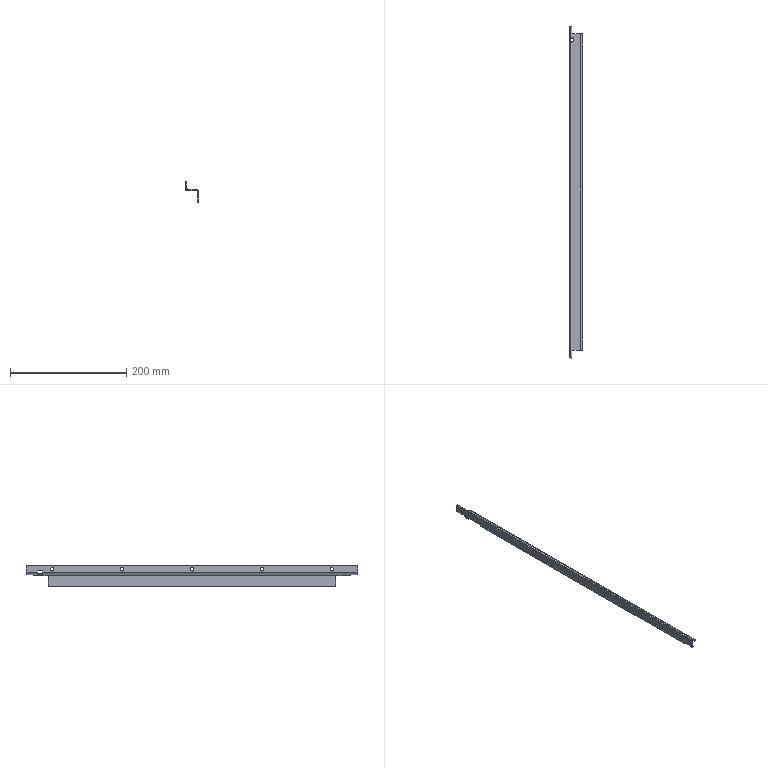Part | NX | features solid 2 | 1 solid | 44 faces | box 22 x 570 x 35 mm | volume 55640 mm3 | plane 26 | cylinder 18 | commonest cylinder face diameters 6 x12 4 x3 8 x3
STEP:
#1=CARTESIAN_POINT('',(-1103.5,-759.5,940.));
#2=VERTEX_POINT('',#1);
#3=CARTESIAN_POINT('',(-1103.5,-759.5,942.));
#4=VERTEX_POINT('',#3);
#5=CARTESIAN_POINT('',(-1103.5,-759.5,940.));
#6=DIRECTION('',(0.,0.,1.));
#7=VECTOR('',#6,1000.);
#8=LINE('',#5,#7);
#9=EDGE_CURVE('',#2,#4,#8,.T.);
#10=ORIENTED_EDGE('',*,*,#9,.F.);
#11=CARTESIAN_POINT('',(-1103.5,-765.5,940.));
#12=VERTEX_POINT('',#11);
#13=CARTESIAN_POINT('',(-1103.5,-762.5,940.));
#14=DIRECTION('',(0.,0.,1.));
#15=DIRECTION('',(0.,-1.,0.));
#16=AXIS2_PLACEMENT_3D('',#13,#14,#15);
#17=CIRCLE('',#16,3.);
#18=EDGE_CURVE('',#12,#2,#17,.T.);
#19=ORIENTED_EDGE('',*,*,#18,.F.);
#20=CARTESIAN_POINT('',(-1103.5,-765.5,942.));
#21=VERTEX_POINT('',#20);
#22=CARTESIAN_POINT('',(-1103.5,-765.5,940.));
#23=DIRECTION('',(0.,0.,1.));
#24=VECTOR('',#23,1000.);
#25=LINE('',#22,#24);
#26=EDGE_CURVE('',#21,#12,#25,.F.);
#27=ORIENTED_EDGE('',*,*,#26,.F.);
#28=CARTESIAN_POINT('',(-1103.5,-762.5,942.));
#29=DIRECTION('',(0.,0.,1.));
#30=DIRECTION('',(-1.,0.,0.));
#31=AXIS2_PLACEMENT_3D('',#28,#29,#30);
#32=CIRCLE('',#31,3.);
#33=EDGE_CURVE('',#21,#4,#32,.T.);
#34=ORIENTED_EDGE('',*,*,#33,.T.);
#35=EDGE_LOOP('',(#10,#19,#27,#34));
#36=FACE_BOUND('',#35,.T.);
#37=CARTESIAN_POINT('',(-1103.5,-762.5,940.));
#38=DIRECTION('',(0.,0.,1.));
#39=DIRECTION('',(0.,-1.,0.));
#40=AXIS2_PLACEMENT_3D('',#37,#38,#39);
#41=CYLINDRICAL_SURFACE('',#40,3.);
#42=ADVANCED_FACE('',(#36),#41,.F.);
#43=CARTESIAN_POINT('',(-1104.,-758.,940.));
#44=VERTEX_POINT('',#43);
#45=CARTESIAN_POINT('',(-1104.,-758.1,940.));
#46=VERTEX_POINT('',#45);
#47=CARTESIAN_POINT('',(-1104.,-758.1,940.));
#48=DIRECTION('',(0.,-1.,0.));
#49=VECTOR('',#48,1000.);
#50=LINE('',#47,#49);
#51=EDGE_CURVE('',#44,#46,#50,.T.);
#52=ORIENTED_EDGE('',*,*,#51,.T.);
#53=CARTESIAN_POINT('',(-1104.,-758.1,942.));
#54=VERTEX_POINT('',#53);
#55=CARTESIAN_POINT('',(-1104.,-758.1,942.));
#56=DIRECTION('',(0.,0.,-1.));
#57=VECTOR('',#56,1000.);
#58=LINE('',#55,#57);
#59=EDGE_CURVE('',#54,#46,#58,.T.);
#60=ORIENTED_EDGE('',*,*,#59,.F.);
#61=CARTESIAN_POINT('',(-1104.,-758.,942.));
#62=VERTEX_POINT('',#61);
#63=CARTESIAN_POINT('',(-1104.,-758.1,942.));
#64=DIRECTION('',(0.,-1.,0.));
#65=VECTOR('',#64,1000.);
#66=LINE('',#63,#65);
#67=EDGE_CURVE('',#62,#54,#66,.T.);
#68=ORIENTED_EDGE('',*,*,#67,.F.);
#69=CARTESIAN_POINT('',(-1104.,-758.,942.));
#70=DIRECTION('',(0.,0.,-1.));
#71=VECTOR('',#70,1000.);
#72=LINE('',#69,#71);
#73=EDGE_CURVE('',#62,#44,#72,.T.);
#74=ORIENTED_EDGE('',*,*,#73,.T.);
#75=EDGE_LOOP('',(#52,#60,#68,#74));
#76=FACE_BOUND('',#75,.T.);
#77=CARTESIAN_POINT('',(-1104.,-758.1,942.));
#78=DIRECTION('',(1.,0.,0.));
#79=DIRECTION('',(0.,0.,-1.));
#80=AXIS2_PLACEMENT_3D('',#77,#78,#79);
#81=PLANE('',#80);
#82=ADVANCED_FACE('',(#76),#81,.F.);
#83=CARTESIAN_POINT('',(-1104.,-767.9,940.));
#84=VERTEX_POINT('',#83);
#85=CARTESIAN_POINT('',(-1104.,-768.,940.));
#86=VERTEX_POINT('',#85);
#87=CARTESIAN_POINT('',(-1104.,-768.,940.));
#88=DIRECTION('',(0.,-1.,0.));
#89=VECTOR('',#88,1000.);
#90=LINE('',#87,#89);
#91=EDGE_CURVE('',#84,#86,#90,.T.);
#92=ORIENTED_EDGE('',*,*,#91,.T.);
#93=CARTESIAN_POINT('',(-1104.,-768.,942.));
#94=VERTEX_POINT('',#93);
#95=CARTESIAN_POINT('',(-1104.,-768.,942.));
#96=DIRECTION('',(0.,0.,-1.));
#97=VECTOR('',#96,1000.);
#98=LINE('',#95,#97);
#99=EDGE_CURVE('',#94,#86,#98,.T.);
#100=ORIENTED_EDGE('',*,*,#99,.F.);
#101=CARTESIAN_POINT('',(-1104.,-767.9,942.));
#102=VERTEX_POINT('',#101);
#103=CARTESIAN_POINT('',(-1104.,-768.,942.));
#104=DIRECTION('',(0.,-1.,0.));
#105=VECTOR('',#104,1000.);
#106=LINE('',#103,#105);
#107=EDGE_CURVE('',#102,#94,#106,.T.);
#108=ORIENTED_EDGE('',*,*,#107,.F.);
#109=CARTESIAN_POINT('',(-1104.,-767.9,942.));
#110=DIRECTION('',(0.,0.,-1.));
#111=VECTOR('',#110,1000.);
#112=LINE('',#109,#111);
#113=EDGE_CURVE('',#102,#84,#112,.T.);
#114=ORIENTED_EDGE('',*,*,#113,.T.);
#115=EDGE_LOOP('',(#92,#100,#108,#114));
#116=FACE_BOUND('',#115,.T.);
#117=CARTESIAN_POINT('',(-1104.,-768.,942.));
#118=DIRECTION('',(1.,0.,0.));
#119=DIRECTION('',(0.,0.,-1.));
#120=AXIS2_PLACEMENT_3D('',#117,#118,#119);
#121=PLANE('',#120);
#122=ADVANCED_FACE('',(#116),#121,.F.);
#123=CARTESIAN_POINT('',(-1108.,-767.9,940.));
#124=VERTEX_POINT('',#123);
#125=CARTESIAN_POINT('',(-1108.,-767.9,940.));
#126=DIRECTION('',(1.,0.,0.));
#127=VECTOR('',#126,1000.);
#128=LINE('',#125,#127);
#129=EDGE_CURVE('',#124,#84,#128,.T.);
#130=ORIENTED_EDGE('',*,*,#129,.T.);
#131=ORIENTED_EDGE('',*,*,#113,.F.);
#132=CARTESIAN_POINT('',(-1108.,-767.9,942.));
#133=VERTEX_POINT('',#132);
#134=CARTESIAN_POINT('',(-1108.,-767.9,942.));
#135=DIRECTION('',(1.,0.,0.));
#136=VECTOR('',#135,1000.);
#137=LINE('',#134,#136);
#138=EDGE_CURVE('',#133,#102,#137,.T.);
#139=ORIENTED_EDGE('',*,*,#138,.F.);
#140=CARTESIAN_POINT('',(-1108.,-767.9,942.));
#141=DIRECTION('',(0.,0.,-1.));
#142=VECTOR('',#141,1000.);
#143=LINE('',#140,#142);
#144=EDGE_CURVE('',#133,#124,#143,.T.);
#145=ORIENTED_EDGE('',*,*,#144,.T.);
#146=EDGE_LOOP('',(#130,#131,#139,#145));
#147=FACE_BOUND('',#146,.T.);
#148=CARTESIAN_POINT('',(-1108.,-767.9,942.));
#149=DIRECTION('',(0.,1.,0.));
#150=DIRECTION('',(0.,0.,-1.));
#151=AXIS2_PLACEMENT_3D('',#148,#149,#150);
#152=PLANE('',#151);
#153=ADVANCED_FACE('',(#147),#152,.F.);
#154=CARTESIAN_POINT('',(-1108.,-758.1,940.));
#155=VERTEX_POINT('',#154);
#156=CARTESIAN_POINT('',(-1108.,-758.1,940.));
#157=DIRECTION('',(0.,-1.,0.));
#158=VECTOR('',#157,1000.);
#159=LINE('',#156,#158);
#160=EDGE_CURVE('',#155,#124,#159,.T.);
#161=ORIENTED_EDGE('',*,*,#160,.T.);
#162=ORIENTED_EDGE('',*,*,#144,.F.);
#163=CARTESIAN_POINT('',(-1108.,-758.1,942.));
#164=VERTEX_POINT('',#163);
#165=CARTESIAN_POINT('',(-1108.,-758.1,942.));
#166=DIRECTION('',(0.,-1.,0.));
#167=VECTOR('',#166,1000.);
#168=LINE('',#165,#167);
#169=EDGE_CURVE('',#164,#133,#168,.T.);
#170=ORIENTED_EDGE('',*,*,#169,.F.);
#171=CARTESIAN_POINT('',(-1108.,-758.1,942.));
#172=DIRECTION('',(0.,0.,-1.));
#173=VECTOR('',#172,1000.);
#174=LINE('',#171,#173);
#175=EDGE_CURVE('',#164,#155,#174,.T.);
#176=ORIENTED_EDGE('',*,*,#175,.T.);
#177=EDGE_LOOP('',(#161,#162,#170,#176));
#178=FACE_BOUND('',#177,.T.);
#179=CARTESIAN_POINT('',(-1108.,-758.1,942.));
#180=DIRECTION('',(1.,0.,0.));
#181=DIRECTION('',(0.,0.,-1.));
#182=AXIS2_PLACEMENT_3D('',#179,#180,#181);
#183=PLANE('',#182);
#184=ADVANCED_FACE('',(#178),#183,.F.);
#185=CARTESIAN_POINT('',(-1104.,-758.1,940.));
#186=DIRECTION('',(-1.,0.,0.));
#187=VECTOR('',#186,1000.);
#188=LINE('',#185,#187);
#189=EDGE_CURVE('',#46,#155,#188,.T.);
#190=ORIENTED_EDGE('',*,*,#189,.T.);
#191=ORIENTED_EDGE('',*,*,#175,.F.);
#192=CARTESIAN_POINT('',(-1104.,-758.1,942.));
#193=DIRECTION('',(-1.,0.,0.));
#194=VECTOR('',#193,1000.);
#195=LINE('',#192,#194);
#196=EDGE_CURVE('',#54,#164,#195,.T.);
#197=ORIENTED_EDGE('',*,*,#196,.F.);
#198=ORIENTED_EDGE('',*,*,#59,.T.);
#199=EDGE_LOOP('',(#190,#191,#197,#198));
#200=FACE_BOUND('',#199,.T.);
#201=CARTESIAN_POINT('',(-1104.,-758.1,942.));
#202=DIRECTION('',(0.,-1.,0.));
#203=DIRECTION('',(-1.,0.,0.));
#204=AXIS2_PLACEMENT_3D('',#201,#202,#203);
#205=PLANE('',#204);
#206=ADVANCED_FACE('',(#200),#205,.F.);
#207=CARTESIAN_POINT('',(-1106.,-768.,947.));
#208=VERTEX_POINT('',#207);
#209=CARTESIAN_POINT('',(-1108.,-768.,947.));
#210=VERTEX_POINT('',#209);
#211=CARTESIAN_POINT('',(-1108.,-768.,947.));
#212=DIRECTION('',(-1.,0.,0.));
#213=VECTOR('',#212,1000.);
#214=LINE('',#211,#213);
#215=EDGE_CURVE('',#208,#210,#214,.T.);
#216=ORIENTED_EDGE('',*,*,#215,.T.);
#217=CARTESIAN_POINT('',(-1108.,-758.,947.));
#218=VERTEX_POINT('',#217);
#219=CARTESIAN_POINT('',(-1108.,-1309.,947.));
#220=DIRECTION('',(0.,1.,0.));
#221=VECTOR('',#220,1000.);
#222=LINE('',#219,#221);
#223=EDGE_CURVE('',#210,#218,#222,.T.);
#224=ORIENTED_EDGE('',*,*,#223,.T.);
#225=CARTESIAN_POINT('',(-1106.,-758.,947.));
#226=VERTEX_POINT('',#225);
#227=CARTESIAN_POINT('',(-1108.,-758.,947.));
#228=DIRECTION('',(-1.,0.,0.));
#229=VECTOR('',#228,1000.);
#230=LINE('',#227,#229);
#231=EDGE_CURVE('',#226,#218,#230,.T.);
#232=ORIENTED_EDGE('',*,*,#231,.F.);
#233=CARTESIAN_POINT('',(-1106.,-1309.,947.));
#234=DIRECTION('',(0.,1.,0.));
#235=VECTOR('',#234,1000.);
#236=LINE('',#233,#235);
#237=EDGE_CURVE('',#208,#226,#236,.T.);
#238=ORIENTED_EDGE('',*,*,#237,.F.);
#239=EDGE_LOOP('',(#216,#224,#232,#238));
#240=FACE_BOUND('',#239,.T.);
#241=CARTESIAN_POINT('',(-1108.,-1309.,947.));
#242=DIRECTION('',(0.,0.,-1.));
#243=DIRECTION('',(0.,-1.,0.));
#244=AXIS2_PLACEMENT_3D('',#241,#242,#243);
#245=PLANE('',#244);
#246=ADVANCED_FACE('',(#240),#245,.T.);
#247=CARTESIAN_POINT('',(-1088.,-1296.,938.));
#248=VERTEX_POINT('',#247);
#249=CARTESIAN_POINT('',(-1090.,-1296.,940.));
#250=VERTEX_POINT('',#249);
#251=CARTESIAN_POINT('',(-1090.,-1296.,938.));
#252=DIRECTION('',(0.,-1.,0.));
#253=DIRECTION('',(0.,0.,-1.));
#254=AXIS2_PLACEMENT_3D('',#251,#252,#253);
#255=CIRCLE('',#254,2.);
#256=EDGE_CURVE('',#248,#250,#255,.T.);
#257=ORIENTED_EDGE('',*,*,#256,.F.);
#258=CARTESIAN_POINT('',(-1086.,-1296.,938.));
#259=VERTEX_POINT('',#258);
#260=CARTESIAN_POINT('',(-1088.,-1296.,938.));
#261=DIRECTION('',(-1.,0.,0.));
#262=VECTOR('',#261,1000.);
#263=LINE('',#260,#262);
#264=EDGE_CURVE('',#259,#248,#263,.T.);
#265=ORIENTED_EDGE('',*,*,#264,.F.);
#266=CARTESIAN_POINT('',(-1090.,-1296.,942.));
#267=VERTEX_POINT('',#266);
#268=CARTESIAN_POINT('',(-1090.,-1296.,938.));
#269=DIRECTION('',(0.,-1.,0.));
#270=DIRECTION('',(0.,0.,-1.));
#271=AXIS2_PLACEMENT_3D('',#268,#269,#270);
#272=CIRCLE('',#271,4.);
#273=EDGE_CURVE('',#259,#267,#272,.T.);
#274=ORIENTED_EDGE('',*,*,#273,.T.);
#275=CARTESIAN_POINT('',(-1104.,-1296.,942.));
#276=VERTEX_POINT('',#275);
#277=CARTESIAN_POINT('',(-1108.,-1296.,942.));
#278=DIRECTION('',(-1.,0.,0.));
#279=VECTOR('',#278,1000.);
#280=LINE('',#277,#279);
#281=EDGE_CURVE('',#267,#276,#280,.T.);
#282=ORIENTED_EDGE('',*,*,#281,.T.);
#283=CARTESIAN_POINT('',(-1104.,-1296.,940.));
#284=VERTEX_POINT('',#283);
#285=CARTESIAN_POINT('',(-1104.,-1296.,940.));
#286=DIRECTION('',(0.,0.,-1.));
#287=VECTOR('',#286,1000.);
#288=LINE('',#285,#287);
#289=EDGE_CURVE('',#276,#284,#288,.T.);
#290=ORIENTED_EDGE('',*,*,#289,.T.);
#291=CARTESIAN_POINT('',(-1108.,-1296.,940.));
#292=DIRECTION('',(-1.,0.,0.));
#293=VECTOR('',#292,1000.);
#294=LINE('',#291,#293);
#295=EDGE_CURVE('',#250,#284,#294,.T.);
#296=ORIENTED_EDGE('',*,*,#295,.F.);
#297=EDGE_LOOP('',(#257,#265,#274,#282,#290,#296));
#298=FACE_BOUND('',#297,.T.);
#299=CARTESIAN_POINT('',(-1090.,-1296.,938.));
#300=DIRECTION('',(0.,-1.,0.));
#301=DIRECTION('',(-1.,0.,0.));
#302=AXIS2_PLACEMENT_3D('',#299,#300,#301);
#303=PLANE('',#302);
#304=ADVANCED_FACE('',(#298),#303,.T.);
#305=CARTESIAN_POINT('',(-1104.,-1309.,942.));
#306=VERTEX_POINT('',#305);
#307=CARTESIAN_POINT('',(-1104.,-1309.,940.));
#308=VERTEX_POINT('',#307);
#309=CARTESIAN_POINT('',(-1104.,-1309.,940.));
#310=DIRECTION('',(0.,0.,-1.));
#311=VECTOR('',#310,1000.);
#312=LINE('',#309,#311);
#313=EDGE_CURVE('',#306,#308,#312,.T.);
#314=ORIENTED_EDGE('',*,*,#313,.T.);
#315=CARTESIAN_POINT('',(-1104.,-1309.,940.));
#316=DIRECTION('',(0.,1.,0.));
#317=VECTOR('',#316,1000.);
#318=LINE('',#315,#317);
#319=EDGE_CURVE('',#308,#284,#318,.T.);
#320=ORIENTED_EDGE('',*,*,#319,.T.);
#321=ORIENTED_EDGE('',*,*,#289,.F.);
#322=CARTESIAN_POINT('',(-1104.,-1309.,942.));
#323=DIRECTION('',(0.,1.,0.));
#324=VECTOR('',#323,1000.);
#325=LINE('',#322,#324);
#326=EDGE_CURVE('',#306,#276,#325,.T.);
#327=ORIENTED_EDGE('',*,*,#326,.F.);
#328=EDGE_LOOP('',(#314,#320,#321,#327));
#329=FACE_BOUND('',#328,.T.);
#330=CARTESIAN_POINT('',(-1104.,-1309.,940.));
#331=DIRECTION('',(1.,0.,0.));
#332=DIRECTION('',(0.,0.,-1.));
#333=AXIS2_PLACEMENT_3D('',#330,#331,#332);
#334=PLANE('',#333);
#335=ADVANCED_FACE('',(#329),#334,.T.);
#336=CARTESIAN_POINT('',(-1104.,-752.,942.));
#337=VERTEX_POINT('',#336);
#338=CARTESIAN_POINT('',(-1090.,-752.,942.));
#339=VERTEX_POINT('',#338);
#340=CARTESIAN_POINT('',(-1108.,-752.,942.));
#341=DIRECTION('',(1.,0.,0.));
#342=VECTOR('',#341,1000.);
#343=LINE('',#340,#342);
#344=EDGE_CURVE('',#337,#339,#343,.T.);
#345=ORIENTED_EDGE('',*,*,#344,.T.);
#346=CARTESIAN_POINT('',(-1086.,-752.,938.));
#347=VERTEX_POINT('',#346);
#348=CARTESIAN_POINT('',(-1090.,-752.,938.));
#349=DIRECTION('',(0.,1.,0.));
#350=DIRECTION('',(0.,0.,-1.));
#351=AXIS2_PLACEMENT_3D('',#348,#349,#350);
#352=CIRCLE('',#351,4.);
#353=EDGE_CURVE('',#339,#347,#352,.T.);
#354=ORIENTED_EDGE('',*,*,#353,.T.);
#355=CARTESIAN_POINT('',(-1088.,-752.,938.));
#356=VERTEX_POINT('',#355);
#357=CARTESIAN_POINT('',(-1088.,-752.,938.));
#358=DIRECTION('',(-1.,0.,0.));
#359=VECTOR('',#358,1000.);
#360=LINE('',#357,#359);
#361=EDGE_CURVE('',#347,#356,#360,.T.);
#362=ORIENTED_EDGE('',*,*,#361,.T.);
#363=CARTESIAN_POINT('',(-1090.,-752.,940.));
#364=VERTEX_POINT('',#363);
#365=CARTESIAN_POINT('',(-1090.,-752.,938.));
#366=DIRECTION('',(0.,1.,0.));
#367=DIRECTION('',(0.,0.,1.));
#368=AXIS2_PLACEMENT_3D('',#365,#366,#367);
#369=CIRCLE('',#368,2.);
#370=EDGE_CURVE('',#364,#356,#369,.T.);
#371=ORIENTED_EDGE('',*,*,#370,.F.);
#372=CARTESIAN_POINT('',(-1104.,-752.,940.));
#373=VERTEX_POINT('',#372);
#374=CARTESIAN_POINT('',(-1108.,-752.,940.));
#375=DIRECTION('',(1.,0.,0.));
#376=VECTOR('',#375,1000.);
#377=LINE('',#374,#376);
#378=EDGE_CURVE('',#373,#364,#377,.T.);
#379=ORIENTED_EDGE('',*,*,#378,.F.);
#380=CARTESIAN_POINT('',(-1104.,-752.,940.));
#381=DIRECTION('',(0.,0.,-1.));
#382=VECTOR('',#381,1000.);
#383=LINE('',#380,#382);
#384=EDGE_CURVE('',#337,#373,#383,.T.);
#385=ORIENTED_EDGE('',*,*,#384,.F.);
#386=EDGE_LOOP('',(#345,#354,#362,#371,#379,#385));
#387=FACE_BOUND('',#386,.T.);
#388=CARTESIAN_POINT('',(-1108.,-752.,940.));
#389=DIRECTION('',(0.,-1.,0.));
#390=DIRECTION('',(-1.,0.,0.));
#391=AXIS2_PLACEMENT_3D('',#388,#389,#390);
#392=PLANE('',#391);
#393=ADVANCED_FACE('',(#387),#392,.F.);
#394=ORIENTED_EDGE('',*,*,#384,.T.);
#395=CARTESIAN_POINT('',(-1104.,-739.,940.));
#396=VERTEX_POINT('',#395);
#397=CARTESIAN_POINT('',(-1104.,-1309.,940.));
#398=DIRECTION('',(0.,1.,0.));
#399=VECTOR('',#398,1000.);
#400=LINE('',#397,#399);
#401=EDGE_CURVE('',#373,#396,#400,.T.);
#402=ORIENTED_EDGE('',*,*,#401,.T.);
#403=CARTESIAN_POINT('',(-1104.,-739.,942.));
#404=VERTEX_POINT('',#403);
#405=CARTESIAN_POINT('',(-1104.,-739.,940.));
#406=DIRECTION('',(0.,0.,-1.));
#407=VECTOR('',#406,1000.);
#408=LINE('',#405,#407);
#409=EDGE_CURVE('',#404,#396,#408,.T.);
#410=ORIENTED_EDGE('',*,*,#409,.F.);
#411=CARTESIAN_POINT('',(-1104.,-1309.,942.));
#412=DIRECTION('',(0.,1.,0.));
#413=VECTOR('',#412,1000.);
#414=LINE('',#411,#413);
#415=EDGE_CURVE('',#337,#404,#414,.T.);
#416=ORIENTED_EDGE('',*,*,#415,.F.);
#417=EDGE_LOOP('',(#394,#402,#410,#416));
#418=FACE_BOUND('',#417,.T.);
#419=CARTESIAN_POINT('',(-1104.,-1309.,940.));
#420=DIRECTION('',(1.,0.,0.));
#421=DIRECTION('',(0.,0.,-1.));
#422=AXIS2_PLACEMENT_3D('',#419,#420,#421);
#423=PLANE('',#422);
#424=ADVANCED_FACE('',(#418),#423,.T.);
#425=CARTESIAN_POINT('',(-1108.,-1024.,946.));
#426=VERTEX_POINT('',#425);
#427=CARTESIAN_POINT('',(-1106.,-1024.,946.));
#428=VERTEX_POINT('',#427);
#429=CARTESIAN_POINT('',(-1677.497,-1024.,946.));
#430=DIRECTION('',(1.,0.,0.));
#431=VECTOR('',#430,1000.);
#432=LINE('',#429,#431);
#433=EDGE_CURVE('',#426,#428,#432,.T.);
#434=ORIENTED_EDGE('',*,*,#433,.F.);
#435=CARTESIAN_POINT('',(-1108.,-1024.,952.));
#436=VERTEX_POINT('',#435);
#437=CARTESIAN_POINT('',(-1108.,-1024.,949.));
#438=DIRECTION('',(1.,0.,0.));
#439=DIRECTION('',(0.,0.,1.));
#440=AXIS2_PLACEMENT_3D('',#437,#438,#439);
#441=CIRCLE('',#440,3.);
#442=EDGE_CURVE('',#436,#426,#441,.T.);
#443=ORIENTED_EDGE('',*,*,#442,.F.);
#444=CARTESIAN_POINT('',(-1106.,-1024.,952.));
#445=VERTEX_POINT('',#444);
#446=CARTESIAN_POINT('',(-1677.497,-1024.,952.));
#447=DIRECTION('',(1.,0.,0.));
#448=VECTOR('',#447,1000.);
#449=LINE('',#446,#448);
#450=EDGE_CURVE('',#445,#436,#449,.F.);
#451=ORIENTED_EDGE('',*,*,#450,.F.);
#452=CARTESIAN_POINT('',(-1106.,-1024.,949.));
#453=DIRECTION('',(1.,0.,0.));
#454=DIRECTION('',(0.,1.,0.));
#455=AXIS2_PLACEMENT_3D('',#452,#453,#454);
#456=CIRCLE('',#455,3.);
#457=EDGE_CURVE('',#445,#428,#456,.T.);
#458=ORIENTED_EDGE('',*,*,#457,.T.);
#459=EDGE_LOOP('',(#434,#443,#451,#458));
#460=FACE_BOUND('',#459,.T.);
#461=CARTESIAN_POINT('',(-1677.497,-1024.,949.));
#462=DIRECTION('',(1.,0.,0.));
#463=DIRECTION('',(0.,0.,1.));
#464=AXIS2_PLACEMENT_3D('',#461,#462,#463);
#465=CYLINDRICAL_SURFACE('',#464,3.);
#466=ADVANCED_FACE('',(#460),#465,.F.);
#467=CARTESIAN_POINT('',(-1108.,-1264.,946.));
#468=VERTEX_POINT('',#467);
#469=CARTESIAN_POINT('',(-1106.,-1264.,946.));
#470=VERTEX_POINT('',#469);
#471=CARTESIAN_POINT('',(-1677.497,-1264.,946.));
#472=DIRECTION('',(1.,0.,0.));
#473=VECTOR('',#472,1000.);
#474=LINE('',#471,#473);
#475=EDGE_CURVE('',#468,#470,#474,.T.);
#476=ORIENTED_EDGE('',*,*,#475,.F.);
#477=CARTESIAN_POINT('',(-1108.,-1264.,952.));
#478=VERTEX_POINT('',#477);
#479=CARTESIAN_POINT('',(-1108.,-1264.,949.));
#480=DIRECTION('',(1.,0.,0.));
#481=DIRECTION('',(0.,0.,1.));
#482=AXIS2_PLACEMENT_3D('',#479,#480,#481);
#483=CIRCLE('',#482,3.);
#484=EDGE_CURVE('',#478,#468,#483,.T.);
#485=ORIENTED_EDGE('',*,*,#484,.F.);
#486=CARTESIAN_POINT('',(-1106.,-1264.,952.));
#487=VERTEX_POINT('',#486);
#488=CARTESIAN_POINT('',(-1677.497,-1264.,952.));
#489=DIRECTION('',(1.,0.,0.));
#490=VECTOR('',#489,1000.);
#491=LINE('',#488,#490);
#492=EDGE_CURVE('',#487,#478,#491,.F.);
#493=ORIENTED_EDGE('',*,*,#492,.F.);
#494=CARTESIAN_POINT('',(-1106.,-1264.,949.));
#495=DIRECTION('',(1.,0.,0.));
#496=DIRECTION('',(0.,1.,0.));
#497=AXIS2_PLACEMENT_3D('',#494,#495,#496);
#498=CIRCLE('',#497,3.);
#499=EDGE_CURVE('',#487,#470,#498,.T.);
#500=ORIENTED_EDGE('',*,*,#499,.T.);
#501=EDGE_LOOP('',(#476,#485,#493,#500));
#502=FACE_BOUND('',#501,.T.);
#503=CARTESIAN_POINT('',(-1677.497,-1264.,949.));
#504=DIRECTION('',(1.,0.,0.));
#505=DIRECTION('',(0.,0.,1.));
#506=AXIS2_PLACEMENT_3D('',#503,#504,#505);
#507=CYLINDRICAL_SURFACE('',#506,3.);
#508=ADVANCED_FACE('',(#502),#507,.F.);
#509=CARTESIAN_POINT('',(-1106.,-1144.,946.));
#510=VERTEX_POINT('',#509);
#511=CARTESIAN_POINT('',(-1108.,-1144.,946.));
#512=VERTEX_POINT('',#511);
#513=CARTESIAN_POINT('',(-1677.497,-1144.,946.));
#514=DIRECTION('',(1.,0.,0.));
#515=VECTOR('',#514,1000.);
#516=LINE('',#513,#515);
#517=EDGE_CURVE('',#510,#512,#516,.F.);
#518=ORIENTED_EDGE('',*,*,#517,.T.);
#519=CARTESIAN_POINT('',(-1108.,-1144.,952.));
#520=VERTEX_POINT('',#519);
#521=CARTESIAN_POINT('',(-1108.,-1144.,949.));
#522=DIRECTION('',(1.,0.,0.));
#523=DIRECTION('',(0.,0.,1.));
#524=AXIS2_PLACEMENT_3D('',#521,#522,#523);
#525=CIRCLE('',#524,3.);
#526=EDGE_CURVE('',#520,#512,#525,.T.);
#527=ORIENTED_EDGE('',*,*,#526,.F.);
#528=CARTESIAN_POINT('',(-1106.,-1144.,952.));
#529=VERTEX_POINT('',#528);
#530=CARTESIAN_POINT('',(-1677.497,-1144.,952.));
#531=DIRECTION('',(1.,0.,0.));
#532=VECTOR('',#531,1000.);
#533=LINE('',#530,#532);
#534=EDGE_CURVE('',#520,#529,#533,.T.);
#535=ORIENTED_EDGE('',*,*,#534,.T.);
#536=CARTESIAN_POINT('',(-1106.,-1144.,949.));
#537=DIRECTION('',(1.,0.,0.));
#538=DIRECTION('',(0.,1.,0.));
#539=AXIS2_PLACEMENT_3D('',#536,#537,#538);
#540=CIRCLE('',#539,3.);
#541=EDGE_CURVE('',#529,#510,#540,.T.);
#542=ORIENTED_EDGE('',*,*,#541,.T.);
#543=EDGE_LOOP('',(#518,#527,#535,#542));
#544=FACE_BOUND('',#543,.T.);
#545=CARTESIAN_POINT('',(-1677.497,-1144.,949.));
#546=DIRECTION('',(1.,0.,0.));
#547=DIRECTION('',(0.,0.,1.));
#548=AXIS2_PLACEMENT_3D('',#545,#546,#547);
#549=CYLINDRICAL_SURFACE('',#548,3.);
#550=ADVANCED_FACE('',(#544),#549,.F.);
#551=CARTESIAN_POINT('',(-1108.,-784.,946.));
#552=VERTEX_POINT('',#551);
#553=CARTESIAN_POINT('',(-1106.,-784.,946.));
#554=VERTEX_POINT('',#553);
#555=CARTESIAN_POINT('',(-1677.497,-784.,946.));
#556=DIRECTION('',(1.,0.,0.));
#557=VECTOR('',#556,1000.);
#558=LINE('',#555,#557);
#559=EDGE_CURVE('',#552,#554,#558,.T.);
#560=ORIENTED_EDGE('',*,*,#559,.F.);
#561=CARTESIAN_POINT('',(-1108.,-784.,952.));
#562=VERTEX_POINT('',#561);
#563=CARTESIAN_POINT('',(-1108.,-784.,949.));
#564=DIRECTION('',(1.,0.,0.));
#565=DIRECTION('',(0.,0.,1.));
#566=AXIS2_PLACEMENT_3D('',#563,#564,#565);
#567=CIRCLE('',#566,3.);
#568=EDGE_CURVE('',#562,#552,#567,.T.);
#569=ORIENTED_EDGE('',*,*,#568,.F.);
#570=CARTESIAN_POINT('',(-1106.,-784.,952.));
#571=VERTEX_POINT('',#570);
#572=CARTESIAN_POINT('',(-1677.497,-784.,952.));
#573=DIRECTION('',(1.,0.,0.));
#574=VECTOR('',#573,1000.);
#575=LINE('',#572,#574);
#576=EDGE_CURVE('',#571,#562,#575,.F.);
#577=ORIENTED_EDGE('',*,*,#576,.F.);
#578=CARTESIAN_POINT('',(-1106.,-784.,949.));
#579=DIRECTION('',(1.,0.,0.));
#580=DIRECTION('',(0.,1.,0.));
#581=AXIS2_PLACEMENT_3D('',#578,#579,#580);
#582=CIRCLE('',#581,3.);
#583=EDGE_CURVE('',#571,#554,#582,.T.);
#584=ORIENTED_EDGE('',*,*,#583,.T.);
#585=EDGE_LOOP('',(#560,#569,#577,#584));
#586=FACE_BOUND('',#585,.T.);
#587=CARTESIAN_POINT('',(-1677.497,-784.,949.));
#588=DIRECTION('',(1.,0.,0.));
#589=DIRECTION('',(0.,0.,1.));
#590=AXIS2_PLACEMENT_3D('',#587,#588,#589);
#591=CYLINDRICAL_SURFACE('',#590,3.);
#592=ADVANCED_FACE('',(#586),#591,.F.);
#593=CARTESIAN_POINT('',(-1106.,-904.,946.));
#594=VERTEX_POINT('',#593);
#595=CARTESIAN_POINT('',(-1108.,-904.,946.));
#596=VERTEX_POINT('',#595);
#597=CARTESIAN_POINT('',(-1677.497,-904.,946.));
#598=DIRECTION('',(1.,0.,0.));
#599=VECTOR('',#598,1000.);
#600=LINE('',#597,#599);
#601=EDGE_CURVE('',#594,#596,#600,.F.);
#602=ORIENTED_EDGE('',*,*,#601,.T.);
#603=CARTESIAN_POINT('',(-1108.,-904.,952.));
#604=VERTEX_POINT('',#603);
#605=CARTESIAN_POINT('',(-1108.,-904.,949.));
#606=DIRECTION('',(1.,0.,0.));
#607=DIRECTION('',(0.,0.,1.));
#608=AXIS2_PLACEMENT_3D('',#605,#606,#607);
#609=CIRCLE('',#608,3.);
#610=EDGE_CURVE('',#604,#596,#609,.T.);
#611=ORIENTED_EDGE('',*,*,#610,.F.);
#612=CARTESIAN_POINT('',(-1106.,-904.,952.));
#613=VERTEX_POINT('',#612);
#614=CARTESIAN_POINT('',(-1677.497,-904.,952.));
#615=DIRECTION('',(1.,0.,0.));
#616=VECTOR('',#615,1000.);
#617=LINE('',#614,#616);
#618=EDGE_CURVE('',#604,#613,#617,.T.);
#619=ORIENTED_EDGE('',*,*,#618,.T.);
#620=CARTESIAN_POINT('',(-1106.,-904.,949.));
#621=DIRECTION('',(1.,0.,0.));
#622=DIRECTION('',(0.,1.,0.));
#623=AXIS2_PLACEMENT_3D('',#620,#621,#622);
#624=CIRCLE('',#623,3.);
#625=EDGE_CURVE('',#613,#594,#624,.T.);
#626=ORIENTED_EDGE('',*,*,#625,.T.);
#627=EDGE_LOOP('',(#602,#611,#619,#626));
#628=FACE_BOUND('',#627,.T.);
#629=CARTESIAN_POINT('',(-1677.497,-904.,949.));
#630=DIRECTION('',(1.,0.,0.));
#631=DIRECTION('',(0.,0.,1.));
#632=AXIS2_PLACEMENT_3D('',#629,#630,#631);
#633=CYLINDRICAL_SURFACE('',#632,3.);
#634=ADVANCED_FACE('',(#628),#633,.F.);
#635=CARTESIAN_POINT('',(-1086.,-1271.,938.));
#636=VERTEX_POINT('',#635);
#637=CARTESIAN_POINT('',(-1088.,-1271.,938.));
#638=VERTEX_POINT('',#637);
#639=CARTESIAN_POINT('',(-1088.,-1271.,938.));
#640=DIRECTION('',(-1.,0.,0.));
#641=VECTOR('',#640,1000.);
#642=LINE('',#639,#641);
#643=EDGE_CURVE('',#636,#638,#642,.T.);
#644=ORIENTED_EDGE('',*,*,#643,.T.);
#645=CARTESIAN_POINT('',(-1088.,-1271.,920.));
#646=VERTEX_POINT('',#645);
#647=CARTESIAN_POINT('',(-1088.,-1271.,940.));
#648=DIRECTION('',(0.,0.,1.));
#649=VECTOR('',#648,1000.);
#650=LINE('',#647,#649);
#651=EDGE_CURVE('',#646,#638,#650,.T.);
#652=ORIENTED_EDGE('',*,*,#651,.F.);
#653=CARTESIAN_POINT('',(-1086.,-1271.,920.));
#654=VERTEX_POINT('',#653);
#655=CARTESIAN_POINT('',(-1088.,-1271.,920.));
#656=DIRECTION('',(-1.,0.,0.));
#657=VECTOR('',#656,1000.);
#658=LINE('',#655,#657);
#659=EDGE_CURVE('',#654,#646,#658,.T.);
#660=ORIENTED_EDGE('',*,*,#659,.F.);
#661=CARTESIAN_POINT('',(-1086.,-1271.,940.));
#662=DIRECTION('',(0.,0.,1.));
#663=VECTOR('',#662,1000.);
#664=LINE('',#661,#663);
#665=EDGE_CURVE('',#654,#636,#664,.T.);
#666=ORIENTED_EDGE('',*,*,#665,.T.);
#667=EDGE_LOOP('',(#644,#652,#660,#666));
#668=FACE_BOUND('',#667,.T.);
#669=CARTESIAN_POINT('',(-1088.,-1271.,940.));
#670=DIRECTION('',(0.,1.,0.));
#671=DIRECTION('',(0.,0.,-1.));
#672=AXIS2_PLACEMENT_3D('',#669,#670,#671);
#673=PLANE('',#672);
#674=ADVANCED_FACE('',(#668),#673,.F.);
#675=CARTESIAN_POINT('',(-1086.,-1309.,938.));
#676=DIRECTION('',(0.,1.,0.));
#677=VECTOR('',#676,1000.);
#678=LINE('',#675,#677);
#679=EDGE_CURVE('',#259,#636,#678,.T.);
#680=ORIENTED_EDGE('',*,*,#679,.F.);
#681=ORIENTED_EDGE('',*,*,#264,.T.);
#682=CARTESIAN_POINT('',(-1088.,-1309.,938.));
#683=DIRECTION('',(0.,1.,0.));
#684=VECTOR('',#683,1000.);
#685=LINE('',#682,#684);
#686=EDGE_CURVE('',#248,#638,#685,.T.);
#687=ORIENTED_EDGE('',*,*,#686,.T.);
#688=ORIENTED_EDGE('',*,*,#643,.F.);
#689=EDGE_LOOP('',(#680,#681,#687,#688));
#690=FACE_BOUND('',#689,.T.);
#691=CARTESIAN_POINT('',(-1088.,-1309.,938.));
#692=DIRECTION('',(0.,0.,-1.));
#693=DIRECTION('',(-1.,0.,0.));
#694=AXIS2_PLACEMENT_3D('',#691,#692,#693);
#695=PLANE('',#694);
#696=ADVANCED_FACE('',(#690),#695,.T.);
#697=CARTESIAN_POINT('',(-1086.,-777.,920.));
#698=VERTEX_POINT('',#697);
#699=CARTESIAN_POINT('',(-1086.,-777.,938.));
#700=VERTEX_POINT('',#699);
#701=CARTESIAN_POINT('',(-1086.,-777.,940.));
#702=DIRECTION('',(0.,0.,1.));
#703=VECTOR('',#702,1000.);
#704=LINE('',#701,#703);
#705=EDGE_CURVE('',#698,#700,#704,.T.);
#706=ORIENTED_EDGE('',*,*,#705,.F.);
#707=CARTESIAN_POINT('',(-1088.,-777.,920.));
#708=VERTEX_POINT('',#707);
#709=CARTESIAN_POINT('',(-1088.,-777.,920.));
#710=DIRECTION('',(-1.,0.,0.));
#711=VECTOR('',#710,1000.);
#712=LINE('',#709,#711);
#713=EDGE_CURVE('',#698,#708,#712,.T.);
#714=ORIENTED_EDGE('',*,*,#713,.T.);
#715=CARTESIAN_POINT('',(-1088.,-777.,938.));
#716=VERTEX_POINT('',#715);
#717=CARTESIAN_POINT('',(-1088.,-777.,940.));
#718=DIRECTION('',(0.,0.,1.));
#719=VECTOR('',#718,1000.);
#720=LINE('',#717,#719);
#721=EDGE_CURVE('',#708,#716,#720,.T.);
#722=ORIENTED_EDGE('',*,*,#721,.T.);
#723=CARTESIAN_POINT('',(-1088.,-777.,938.));
#724=DIRECTION('',(-1.,0.,0.));
#725=VECTOR('',#724,1000.);
#726=LINE('',#723,#725);
#727=EDGE_CURVE('',#700,#716,#726,.T.);
#728=ORIENTED_EDGE('',*,*,#727,.F.);
#729=EDGE_LOOP('',(#706,#714,#722,#728));
#730=FACE_BOUND('',#729,.T.);
#731=CARTESIAN_POINT('',(-1088.,-777.,940.));
#732=DIRECTION('',(0.,1.,0.));
#733=DIRECTION('',(0.,0.,-1.));
#734=AXIS2_PLACEMENT_3D('',#731,#732,#733);
#735=PLANE('',#734);
#736=ADVANCED_FACE('',(#730),#735,.T.);
#737=CARTESIAN_POINT('',(-1088.,-1309.,920.));
#738=DIRECTION('',(0.,1.,0.));
#739=VECTOR('',#738,1000.);
#740=LINE('',#737,#739);
#741=EDGE_CURVE('',#646,#708,#740,.T.);
#742=ORIENTED_EDGE('',*,*,#741,.F.);
#743=ORIENTED_EDGE('',*,*,#651,.T.);
#744=CARTESIAN_POINT('',(-1088.,-1309.,938.));
#745=DIRECTION('',(0.,1.,0.));
#746=VECTOR('',#745,1000.);
#747=LINE('',#744,#746);
#748=EDGE_CURVE('',#638,#716,#747,.T.);
#749=ORIENTED_EDGE('',*,*,#748,.T.);
#750=ORIENTED_EDGE('',*,*,#721,.F.);
#751=EDGE_LOOP('',(#742,#743,#749,#750));
#752=FACE_BOUND('',#751,.T.);
#753=CARTESIAN_POINT('',(-1088.,-1309.,940.));
#754=DIRECTION('',(1.,0.,0.));
#755=DIRECTION('',(0.,0.,-1.));
#756=AXIS2_PLACEMENT_3D('',#753,#754,#755);
#757=PLANE('',#756);
#758=ADVANCED_FACE('',(#752),#757,.F.);
#759=ORIENTED_EDGE('',*,*,#686,.F.);
#760=ORIENTED_EDGE('',*,*,#256,.T.);
#761=CARTESIAN_POINT('',(-1090.,-1309.,940.));
#762=DIRECTION('',(0.,1.,0.));
#763=VECTOR('',#762,1000.);
#764=LINE('',#761,#763);
#765=EDGE_CURVE('',#250,#364,#764,.T.);
#766=ORIENTED_EDGE('',*,*,#765,.T.);
#767=ORIENTED_EDGE('',*,*,#370,.T.);
#768=CARTESIAN_POINT('',(-1088.,-1309.,938.));
#769=DIRECTION('',(0.,1.,0.));
#770=VECTOR('',#769,1000.);
#771=LINE('',#768,#770);
#772=EDGE_CURVE('',#716,#356,#771,.T.);
#773=ORIENTED_EDGE('',*,*,#772,.F.);
#774=ORIENTED_EDGE('',*,*,#748,.F.);
#775=EDGE_LOOP('',(#759,#760,#766,#767,#773,#774));
#776=FACE_BOUND('',#775,.T.);
#777=CARTESIAN_POINT('',(-1090.,-1309.,938.));
#778=DIRECTION('',(0.,1.,0.));
#779=DIRECTION('',(0.,0.,-1.));
#780=AXIS2_PLACEMENT_3D('',#777,#778,#779);
#781=CYLINDRICAL_SURFACE('',#780,2.);
#782=ADVANCED_FACE('',(#776),#781,.F.);
#783=ORIENTED_EDGE('',*,*,#18,.T.);
#784=CARTESIAN_POINT('',(-1103.5,-762.5,940.));
#785=DIRECTION('',(0.,0.,1.));
#786=DIRECTION('',(0.,-1.,0.));
#787=AXIS2_PLACEMENT_3D('',#784,#785,#786);
#788=CIRCLE('',#787,3.);
#789=EDGE_CURVE('',#2,#12,#788,.T.);
#790=ORIENTED_EDGE('',*,*,#789,.T.);
#791=EDGE_LOOP('',(#783,#790));
#792=FACE_BOUND('',#791,.T.);
#793=ORIENTED_EDGE('',*,*,#51,.F.);
#794=CARTESIAN_POINT('',(-1104.,-1309.,940.));
#795=DIRECTION('',(0.,1.,0.));
#796=VECTOR('',#795,1000.);
#797=LINE('',#794,#796);
#798=EDGE_CURVE('',#44,#373,#797,.T.);
#799=ORIENTED_EDGE('',*,*,#798,.T.);
#800=ORIENTED_EDGE('',*,*,#378,.T.);
#801=ORIENTED_EDGE('',*,*,#765,.F.);
#802=ORIENTED_EDGE('',*,*,#295,.T.);
#803=CARTESIAN_POINT('',(-1104.,-1309.,940.));
#804=DIRECTION('',(0.,1.,0.));
#805=VECTOR('',#804,1000.);
#806=LINE('',#803,#805);
#807=EDGE_CURVE('',#284,#86,#806,.T.);
#808=ORIENTED_EDGE('',*,*,#807,.T.);
#809=ORIENTED_EDGE('',*,*,#91,.F.);
#810=ORIENTED_EDGE('',*,*,#129,.F.);
#811=ORIENTED_EDGE('',*,*,#160,.F.);
#812=ORIENTED_EDGE('',*,*,#189,.F.);
#813=EDGE_LOOP('',(#793,#799,#800,#801,#802,#808,#809,#810,#811,#812));
#814=FACE_BOUND('',#813,.T.);
#815=CARTESIAN_POINT('',(-1108.,-1309.,940.));
#816=DIRECTION('',(0.,0.,1.));
#817=DIRECTION('',(0.,-1.,0.));
#818=AXIS2_PLACEMENT_3D('',#815,#816,#817);
#819=PLANE('',#818);
#820=ADVANCED_FACE('',(#792,#814),#819,.F.);
#821=CARTESIAN_POINT('',(-1108.,-1309.,944.));
#822=VERTEX_POINT('',#821);
#823=CARTESIAN_POINT('',(-1108.,-768.,944.));
#824=VERTEX_POINT('',#823);
#825=CARTESIAN_POINT('',(-1108.,-1309.,944.));
#826=DIRECTION('',(0.,1.,0.));
#827=VECTOR('',#826,1000.);
#828=LINE('',#825,#827);
#829=EDGE_CURVE('',#822,#824,#828,.T.);
#830=ORIENTED_EDGE('',*,*,#829,.T.);
#831=CARTESIAN_POINT('',(-1104.,-768.,944.));
#832=DIRECTION('',(0.,-1.,0.));
#833=DIRECTION('',(0.,0.,1.));
#834=AXIS2_PLACEMENT_3D('',#831,#832,#833);
#835=CIRCLE('',#834,4.);
#836=EDGE_CURVE('',#824,#86,#835,.T.);
#837=ORIENTED_EDGE('',*,*,#836,.T.);
#838=ORIENTED_EDGE('',*,*,#807,.F.);
#839=ORIENTED_EDGE('',*,*,#319,.F.);
#840=CARTESIAN_POINT('',(-1104.,-1309.,944.));
#841=DIRECTION('',(0.,-1.,0.));
#842=DIRECTION('',(0.,0.,-1.));
#843=AXIS2_PLACEMENT_3D('',#840,#841,#842);
#844=CIRCLE('',#843,4.);
#845=EDGE_CURVE('',#822,#308,#844,.T.);
#846=ORIENTED_EDGE('',*,*,#845,.F.);
#847=EDGE_LOOP('',(#830,#837,#838,#839,#846));
#848=FACE_BOUND('',#847,.T.);
#849=CARTESIAN_POINT('',(-1104.,-1309.,944.));
#850=DIRECTION('',(0.,1.,0.));
#851=DIRECTION('',(0.,0.,-1.));
#852=AXIS2_PLACEMENT_3D('',#849,#850,#851);
#853=CYLINDRICAL_SURFACE('',#852,4.);
#854=ADVANCED_FACE('',(#848),#853,.T.);
#855=ORIENTED_EDGE('',*,*,#610,.T.);
#856=CARTESIAN_POINT('',(-1108.,-904.,949.));
#857=DIRECTION('',(1.,0.,0.));
#858=DIRECTION('',(0.,0.,1.));
#859=AXIS2_PLACEMENT_3D('',#856,#857,#858);
#860=CIRCLE('',#859,3.);
#861=EDGE_CURVE('',#596,#604,#860,.T.);
#862=ORIENTED_EDGE('',*,*,#861,.T.);
#863=EDGE_LOOP('',(#855,#862));
#864=FACE_BOUND('',#863,.T.);
#865=ORIENTED_EDGE('',*,*,#568,.T.);
#866=CARTESIAN_POINT('',(-1108.,-784.,949.));
#867=DIRECTION('',(1.,0.,0.));
#868=DIRECTION('',(0.,0.,1.));
#869=AXIS2_PLACEMENT_3D('',#866,#867,#868);
#870=CIRCLE('',#869,3.);
#871=EDGE_CURVE('',#552,#562,#870,.T.);
#872=ORIENTED_EDGE('',*,*,#871,.T.);
#873=EDGE_LOOP('',(#865,#872));
#874=FACE_BOUND('',#873,.T.);
#875=ORIENTED_EDGE('',*,*,#526,.T.);
#876=CARTESIAN_POINT('',(-1108.,-1144.,949.));
#877=DIRECTION('',(1.,0.,0.));
#878=DIRECTION('',(0.,0.,1.));
#879=AXIS2_PLACEMENT_3D('',#876,#877,#878);
#880=CIRCLE('',#879,3.);
#881=EDGE_CURVE('',#512,#520,#880,.T.);
#882=ORIENTED_EDGE('',*,*,#881,.T.);
#883=EDGE_LOOP('',(#875,#882));
#884=FACE_BOUND('',#883,.T.);
#885=ORIENTED_EDGE('',*,*,#484,.T.);
#886=CARTESIAN_POINT('',(-1108.,-1264.,949.));
#887=DIRECTION('',(1.,0.,0.));
#888=DIRECTION('',(0.,0.,1.));
#889=AXIS2_PLACEMENT_3D('',#886,#887,#888);
#890=CIRCLE('',#889,3.);
#891=EDGE_CURVE('',#468,#478,#890,.T.);
#892=ORIENTED_EDGE('',*,*,#891,.T.);
#893=EDGE_LOOP('',(#885,#892));
#894=FACE_BOUND('',#893,.T.);
#895=ORIENTED_EDGE('',*,*,#442,.T.);
#896=CARTESIAN_POINT('',(-1108.,-1024.,949.));
#897=DIRECTION('',(1.,0.,0.));
#898=DIRECTION('',(0.,0.,1.));
#899=AXIS2_PLACEMENT_3D('',#896,#897,#898);
#900=CIRCLE('',#899,3.);
#901=EDGE_CURVE('',#426,#436,#900,.T.);
#902=ORIENTED_EDGE('',*,*,#901,.T.);
#903=EDGE_LOOP('',(#895,#902));
#904=FACE_BOUND('',#903,.T.);
#905=CARTESIAN_POINT('',(-1108.,-758.,944.));
#906=VERTEX_POINT('',#905);
#907=CARTESIAN_POINT('',(-1108.,-739.,944.));
#908=VERTEX_POINT('',#907);
#909=CARTESIAN_POINT('',(-1108.,-1309.,944.));
#910=DIRECTION('',(0.,1.,0.));
#911=VECTOR('',#910,1000.);
#912=LINE('',#909,#911);
#913=EDGE_CURVE('',#906,#908,#912,.T.);
#914=ORIENTED_EDGE('',*,*,#913,.F.);
#915=CARTESIAN_POINT('',(-1108.,-758.,955.));
#916=DIRECTION('',(0.,0.,1.));
#917=VECTOR('',#916,1000.);
#918=LINE('',#915,#917);
#919=EDGE_CURVE('',#906,#218,#918,.T.);
#920=ORIENTED_EDGE('',*,*,#919,.T.);
#921=ORIENTED_EDGE('',*,*,#223,.F.);
#922=CARTESIAN_POINT('',(-1108.,-768.,955.));
#923=DIRECTION('',(0.,0.,-1.));
#924=VECTOR('',#923,1000.);
#925=LINE('',#922,#924);
#926=EDGE_CURVE('',#210,#824,#925,.T.);
#927=ORIENTED_EDGE('',*,*,#926,.T.);
#928=ORIENTED_EDGE('',*,*,#829,.F.);
#929=CARTESIAN_POINT('',(-1108.,-1309.,955.));
#930=VERTEX_POINT('',#929);
#931=CARTESIAN_POINT('',(-1108.,-1309.,955.));
#932=DIRECTION('',(0.,0.,-1.));
#933=VECTOR('',#932,1000.);
#934=LINE('',#931,#933);
#935=EDGE_CURVE('',#930,#822,#934,.T.);
#936=ORIENTED_EDGE('',*,*,#935,.F.);
#937=CARTESIAN_POINT('',(-1108.,-739.,955.));
#938=VERTEX_POINT('',#937);
#939=CARTESIAN_POINT('',(-1108.,-1309.,955.));
#940=DIRECTION('',(0.,1.,0.));
#941=VECTOR('',#940,1000.);
#942=LINE('',#939,#941);
#943=EDGE_CURVE('',#930,#938,#942,.T.);
#944=ORIENTED_EDGE('',*,*,#943,.T.);
#945=CARTESIAN_POINT('',(-1108.,-739.,955.));
#946=DIRECTION('',(0.,0.,-1.));
#947=VECTOR('',#946,1000.);
#948=LINE('',#945,#947);
#949=EDGE_CURVE('',#938,#908,#948,.T.);
#950=ORIENTED_EDGE('',*,*,#949,.T.);
#951=EDGE_LOOP('',(#914,#920,#921,#927,#928,#936,#944,#950));
#952=FACE_BOUND('',#951,.T.);
#953=CARTESIAN_POINT('',(-1108.,-1309.,955.));
#954=DIRECTION('',(1.,0.,0.));
#955=DIRECTION('',(0.,0.,-1.));
#956=AXIS2_PLACEMENT_3D('',#953,#954,#955);
#957=PLANE('',#956);
#958=ADVANCED_FACE('',(#864,#874,#884,#894,#904,#952),#957,.F.);
#959=ORIENTED_EDGE('',*,*,#665,.F.);
#960=CARTESIAN_POINT('',(-1086.,-1309.,920.));
#961=DIRECTION('',(0.,1.,0.));
#962=VECTOR('',#961,1000.);
#963=LINE('',#960,#962);
#964=EDGE_CURVE('',#654,#698,#963,.T.);
#965=ORIENTED_EDGE('',*,*,#964,.T.);
#966=ORIENTED_EDGE('',*,*,#705,.T.);
#967=CARTESIAN_POINT('',(-1086.,-1309.,938.));
#968=DIRECTION('',(0.,1.,0.));
#969=VECTOR('',#968,1000.);
#970=LINE('',#967,#969);
#971=EDGE_CURVE('',#636,#700,#970,.T.);
#972=ORIENTED_EDGE('',*,*,#971,.F.);
#973=EDGE_LOOP('',(#959,#965,#966,#972));
#974=FACE_BOUND('',#973,.T.);
#975=CARTESIAN_POINT('',(-1086.,-1309.,940.));
#976=DIRECTION('',(1.,0.,0.));
#977=DIRECTION('',(0.,0.,-1.));
#978=AXIS2_PLACEMENT_3D('',#975,#976,#977);
#979=PLANE('',#978);
#980=ADVANCED_FACE('',(#974),#979,.T.);
#981=ORIENTED_EDGE('',*,*,#273,.F.);
#982=ORIENTED_EDGE('',*,*,#679,.T.);
#983=ORIENTED_EDGE('',*,*,#971,.T.);
#984=CARTESIAN_POINT('',(-1086.,-1309.,938.));
#985=DIRECTION('',(0.,1.,0.));
#986=VECTOR('',#985,1000.);
#987=LINE('',#984,#986);
#988=EDGE_CURVE('',#700,#347,#987,.T.);
#989=ORIENTED_EDGE('',*,*,#988,.T.);
#990=ORIENTED_EDGE('',*,*,#353,.F.);
#991=CARTESIAN_POINT('',(-1090.,-1309.,942.));
#992=DIRECTION('',(0.,1.,0.));
#993=VECTOR('',#992,1000.);
#994=LINE('',#991,#993);
#995=EDGE_CURVE('',#267,#339,#994,.T.);
#996=ORIENTED_EDGE('',*,*,#995,.F.);
#997=EDGE_LOOP('',(#981,#982,#983,#989,#990,#996));
#998=FACE_BOUND('',#997,.T.);
#999=CARTESIAN_POINT('',(-1090.,-1309.,938.));
#1000=DIRECTION('',(0.,1.,0.));
#1001=DIRECTION('',(0.,0.,-1.));
#1002=AXIS2_PLACEMENT_3D('',#999,#1000,#1001);
#1003=CYLINDRICAL_SURFACE('',#1002,4.);
#1004=ADVANCED_FACE('',(#998),#1003,.T.);
#1005=ORIENTED_EDGE('',*,*,#33,.F.);
#1006=CARTESIAN_POINT('',(-1103.5,-762.5,942.));
#1007=DIRECTION('',(0.,0.,1.));
#1008=DIRECTION('',(-1.,0.,0.));
#1009=AXIS2_PLACEMENT_3D('',#1006,#1007,#1008);
#1010=CIRCLE('',#1009,3.);
#1011=EDGE_CURVE('',#4,#21,#1010,.T.);
#1012=ORIENTED_EDGE('',*,*,#1011,.F.);
#1013=EDGE_LOOP('',(#1005,#1012));
#1014=FACE_BOUND('',#1013,.T.);
#1015=CARTESIAN_POINT('',(-1104.,-1309.,942.));
#1016=DIRECTION('',(0.,1.,0.));
#1017=VECTOR('',#1016,1000.);
#1018=LINE('',#1015,#1017);
#1019=EDGE_CURVE('',#62,#337,#1018,.T.);
#1020=ORIENTED_EDGE('',*,*,#1019,.F.);
#1021=ORIENTED_EDGE('',*,*,#67,.T.);
#1022=ORIENTED_EDGE('',*,*,#196,.T.);
#1023=ORIENTED_EDGE('',*,*,#169,.T.);
#1024=ORIENTED_EDGE('',*,*,#138,.T.);
#1025=ORIENTED_EDGE('',*,*,#107,.T.);
#1026=CARTESIAN_POINT('',(-1104.,-1309.,942.));
#1027=DIRECTION('',(0.,1.,0.));
#1028=VECTOR('',#1027,1000.);
#1029=LINE('',#1026,#1028);
#1030=EDGE_CURVE('',#276,#94,#1029,.T.);
#1031=ORIENTED_EDGE('',*,*,#1030,.F.);
#1032=ORIENTED_EDGE('',*,*,#281,.F.);
#1033=ORIENTED_EDGE('',*,*,#995,.T.);
#1034=ORIENTED_EDGE('',*,*,#344,.F.);
#1035=EDGE_LOOP('',(#1020,#1021,#1022,#1023,#1024,#1025,#1031,#1032,#1033,#1034));
#1036=FACE_BOUND('',#1035,.T.);
#1037=CARTESIAN_POINT('',(-1108.,-1309.,942.));
#1038=DIRECTION('',(0.,0.,1.));
#1039=DIRECTION('',(0.,-1.,0.));
#1040=AXIS2_PLACEMENT_3D('',#1037,#1038,#1039);
#1041=PLANE('',#1040);
#1042=ADVANCED_FACE('',(#1014,#1036),#1041,.T.);
#1043=CARTESIAN_POINT('',(-1106.,-768.,944.));
#1044=VERTEX_POINT('',#1043);
#1045=CARTESIAN_POINT('',(-1104.,-768.,944.));
#1046=DIRECTION('',(0.,-1.,0.));
#1047=DIRECTION('',(0.,0.,-1.));
#1048=AXIS2_PLACEMENT_3D('',#1045,#1046,#1047);
#1049=CIRCLE('',#1048,2.);
#1050=EDGE_CURVE('',#1044,#94,#1049,.T.);
#1051=ORIENTED_EDGE('',*,*,#1050,.F.);
#1052=CARTESIAN_POINT('',(-1106.,-1309.,944.));
#1053=VERTEX_POINT('',#1052);
#1054=CARTESIAN_POINT('',(-1106.,-1309.,944.));
#1055=DIRECTION('',(0.,1.,0.));
#1056=VECTOR('',#1055,1000.);
#1057=LINE('',#1054,#1056);
#1058=EDGE_CURVE('',#1053,#1044,#1057,.T.);
#1059=ORIENTED_EDGE('',*,*,#1058,.F.);
#1060=CARTESIAN_POINT('',(-1104.,-1309.,944.));
#1061=DIRECTION('',(0.,-1.,0.));
#1062=DIRECTION('',(0.,0.,-1.));
#1063=AXIS2_PLACEMENT_3D('',#1060,#1061,#1062);
#1064=CIRCLE('',#1063,2.);
#1065=EDGE_CURVE('',#1053,#306,#1064,.T.);
#1066=ORIENTED_EDGE('',*,*,#1065,.T.);
#1067=ORIENTED_EDGE('',*,*,#326,.T.);
#1068=ORIENTED_EDGE('',*,*,#1030,.T.);
#1069=EDGE_LOOP('',(#1051,#1059,#1066,#1067,#1068));
#1070=FACE_BOUND('',#1069,.T.);
#1071=CARTESIAN_POINT('',(-1104.,-1309.,944.));
#1072=DIRECTION('',(0.,1.,0.));
#1073=DIRECTION('',(0.,0.,-1.));
#1074=AXIS2_PLACEMENT_3D('',#1071,#1072,#1073);
#1075=CYLINDRICAL_SURFACE('',#1074,2.);
#1076=ADVANCED_FACE('',(#1070),#1075,.F.);
#1077=ORIENTED_EDGE('',*,*,#625,.F.);
#1078=CARTESIAN_POINT('',(-1106.,-904.,949.));
#1079=DIRECTION('',(1.,0.,0.));
#1080=DIRECTION('',(0.,1.,0.));
#1081=AXIS2_PLACEMENT_3D('',#1078,#1079,#1080);
#1082=CIRCLE('',#1081,3.);
#1083=EDGE_CURVE('',#594,#613,#1082,.T.);
#1084=ORIENTED_EDGE('',*,*,#1083,.F.);
#1085=EDGE_LOOP('',(#1077,#1084));
#1086=FACE_BOUND('',#1085,.T.);
#1087=ORIENTED_EDGE('',*,*,#583,.F.);
#1088=CARTESIAN_POINT('',(-1106.,-784.,949.));
#1089=DIRECTION('',(1.,0.,0.));
#1090=DIRECTION('',(0.,1.,0.));
#1091=AXIS2_PLACEMENT_3D('',#1088,#1089,#1090);
#1092=CIRCLE('',#1091,3.);
#1093=EDGE_CURVE('',#554,#571,#1092,.T.);
#1094=ORIENTED_EDGE('',*,*,#1093,.F.);
#1095=EDGE_LOOP('',(#1087,#1094));
#1096=FACE_BOUND('',#1095,.T.);
#1097=ORIENTED_EDGE('',*,*,#541,.F.);
#1098=CARTESIAN_POINT('',(-1106.,-1144.,949.));
#1099=DIRECTION('',(1.,0.,0.));
#1100=DIRECTION('',(0.,1.,0.));
#1101=AXIS2_PLACEMENT_3D('',#1098,#1099,#1100);
#1102=CIRCLE('',#1101,3.);
#1103=EDGE_CURVE('',#510,#529,#1102,.T.);
#1104=ORIENTED_EDGE('',*,*,#1103,.F.);
#1105=EDGE_LOOP('',(#1097,#1104));
#1106=FACE_BOUND('',#1105,.T.);
#1107=ORIENTED_EDGE('',*,*,#499,.F.);
#1108=CARTESIAN_POINT('',(-1106.,-1264.,949.));
#1109=DIRECTION('',(1.,0.,0.));
#1110=DIRECTION('',(0.,1.,0.));
#1111=AXIS2_PLACEMENT_3D('',#1108,#1109,#1110);
#1112=CIRCLE('',#1111,3.);
#1113=EDGE_CURVE('',#470,#487,#1112,.T.);
#1114=ORIENTED_EDGE('',*,*,#1113,.F.);
#1115=EDGE_LOOP('',(#1107,#1114));
#1116=FACE_BOUND('',#1115,.T.);
#1117=ORIENTED_EDGE('',*,*,#457,.F.);
#1118=CARTESIAN_POINT('',(-1106.,-1024.,949.));
#1119=DIRECTION('',(1.,0.,0.));
#1120=DIRECTION('',(0.,1.,0.));
#1121=AXIS2_PLACEMENT_3D('',#1118,#1119,#1120);
#1122=CIRCLE('',#1121,3.);
#1123=EDGE_CURVE('',#428,#445,#1122,.T.);
#1124=ORIENTED_EDGE('',*,*,#1123,.F.);
#1125=EDGE_LOOP('',(#1117,#1124));
#1126=FACE_BOUND('',#1125,.T.);
#1127=CARTESIAN_POINT('',(-1106.,-758.,944.));
#1128=VERTEX_POINT('',#1127);
#1129=CARTESIAN_POINT('',(-1106.,-758.,955.));
#1130=DIRECTION('',(0.,0.,1.));
#1131=VECTOR('',#1130,1000.);
#1132=LINE('',#1129,#1131);
#1133=EDGE_CURVE('',#1128,#226,#1132,.T.);
#1134=ORIENTED_EDGE('',*,*,#1133,.F.);
#1135=CARTESIAN_POINT('',(-1106.,-739.,944.));
#1136=VERTEX_POINT('',#1135);
#1137=CARTESIAN_POINT('',(-1106.,-1309.,944.));
#1138=DIRECTION('',(0.,1.,0.));
#1139=VECTOR('',#1138,1000.);
#1140=LINE('',#1137,#1139);
#1141=EDGE_CURVE('',#1128,#1136,#1140,.T.);
#1142=ORIENTED_EDGE('',*,*,#1141,.T.);
#1143=CARTESIAN_POINT('',(-1106.,-739.,955.));
#1144=VERTEX_POINT('',#1143);
#1145=CARTESIAN_POINT('',(-1106.,-739.,955.));
#1146=DIRECTION('',(0.,0.,-1.));
#1147=VECTOR('',#1146,1000.);
#1148=LINE('',#1145,#1147);
#1149=EDGE_CURVE('',#1144,#1136,#1148,.T.);
#1150=ORIENTED_EDGE('',*,*,#1149,.F.);
#1151=CARTESIAN_POINT('',(-1106.,-1309.,955.));
#1152=VERTEX_POINT('',#1151);
#1153=CARTESIAN_POINT('',(-1106.,-1309.,955.));
#1154=DIRECTION('',(0.,1.,0.));
#1155=VECTOR('',#1154,1000.);
#1156=LINE('',#1153,#1155);
#1157=EDGE_CURVE('',#1152,#1144,#1156,.T.);
#1158=ORIENTED_EDGE('',*,*,#1157,.F.);
#1159=CARTESIAN_POINT('',(-1106.,-1309.,955.));
#1160=DIRECTION('',(0.,0.,-1.));
#1161=VECTOR('',#1160,1000.);
#1162=LINE('',#1159,#1161);
#1163=EDGE_CURVE('',#1152,#1053,#1162,.T.);
#1164=ORIENTED_EDGE('',*,*,#1163,.T.);
#1165=ORIENTED_EDGE('',*,*,#1058,.T.);
#1166=CARTESIAN_POINT('',(-1106.,-768.,955.));
#1167=DIRECTION('',(0.,0.,-1.));
#1168=VECTOR('',#1167,1000.);
#1169=LINE('',#1166,#1168);
#1170=EDGE_CURVE('',#208,#1044,#1169,.T.);
#1171=ORIENTED_EDGE('',*,*,#1170,.F.);
#1172=ORIENTED_EDGE('',*,*,#237,.T.);
#1173=EDGE_LOOP('',(#1134,#1142,#1150,#1158,#1164,#1165,#1171,#1172));
#1174=FACE_BOUND('',#1173,.T.);
#1175=CARTESIAN_POINT('',(-1106.,-1309.,955.));
#1176=DIRECTION('',(1.,0.,0.));
#1177=DIRECTION('',(0.,0.,-1.));
#1178=AXIS2_PLACEMENT_3D('',#1175,#1176,#1177);
#1179=PLANE('',#1178);
#1180=ADVANCED_FACE('',(#1086,#1096,#1106,#1116,#1126,#1174),#1179,.T.);
#1181=ORIENTED_EDGE('',*,*,#943,.F.);
#1182=CARTESIAN_POINT('',(-1108.,-1309.,955.));
#1183=DIRECTION('',(1.,0.,0.));
#1184=VECTOR('',#1183,1000.);
#1185=LINE('',#1182,#1184);
#1186=EDGE_CURVE('',#930,#1152,#1185,.T.);
#1187=ORIENTED_EDGE('',*,*,#1186,.T.);
#1188=ORIENTED_EDGE('',*,*,#1157,.T.);
#1189=CARTESIAN_POINT('',(-1108.,-739.,955.));
#1190=DIRECTION('',(1.,0.,0.));
#1191=VECTOR('',#1190,1000.);
#1192=LINE('',#1189,#1191);
#1193=EDGE_CURVE('',#938,#1144,#1192,.T.);
#1194=ORIENTED_EDGE('',*,*,#1193,.F.);
#1195=EDGE_LOOP('',(#1181,#1187,#1188,#1194));
#1196=FACE_BOUND('',#1195,.T.);
#1197=CARTESIAN_POINT('',(-1108.,-1309.,955.));
#1198=DIRECTION('',(0.,0.,-1.));
#1199=DIRECTION('',(0.,-1.,0.));
#1200=AXIS2_PLACEMENT_3D('',#1197,#1198,#1199);
#1201=PLANE('',#1200);
#1202=ADVANCED_FACE('',(#1196),#1201,.F.);
#1203=ORIENTED_EDGE('',*,*,#313,.F.);
#1204=ORIENTED_EDGE('',*,*,#1065,.F.);
#1205=ORIENTED_EDGE('',*,*,#1163,.F.);
#1206=ORIENTED_EDGE('',*,*,#1186,.F.);
#1207=ORIENTED_EDGE('',*,*,#935,.T.);
#1208=ORIENTED_EDGE('',*,*,#845,.T.);
#1209=EDGE_LOOP('',(#1203,#1204,#1205,#1206,#1207,#1208));
#1210=FACE_BOUND('',#1209,.T.);
#1211=CARTESIAN_POINT('',(-1088.,-1309.,940.));
#1212=DIRECTION('',(0.,-1.,0.));
#1213=DIRECTION('',(-1.,0.,0.));
#1214=AXIS2_PLACEMENT_3D('',#1211,#1212,#1213);
#1215=PLANE('',#1214);
#1216=ADVANCED_FACE('',(#1210),#1215,.T.);
#1217=ORIENTED_EDGE('',*,*,#964,.F.);
#1218=ORIENTED_EDGE('',*,*,#659,.T.);
#1219=ORIENTED_EDGE('',*,*,#741,.T.);
#1220=ORIENTED_EDGE('',*,*,#713,.F.);
#1221=EDGE_LOOP('',(#1217,#1218,#1219,#1220));
#1222=FACE_BOUND('',#1221,.T.);
#1223=CARTESIAN_POINT('',(-1088.,-1309.,920.));
#1224=DIRECTION('',(0.,0.,-1.));
#1225=DIRECTION('',(-1.,0.,0.));
#1226=AXIS2_PLACEMENT_3D('',#1223,#1224,#1225);
#1227=PLANE('',#1226);
#1228=ADVANCED_FACE('',(#1222),#1227,.T.);
#1229=ORIENTED_EDGE('',*,*,#361,.F.);
#1230=ORIENTED_EDGE('',*,*,#988,.F.);
#1231=ORIENTED_EDGE('',*,*,#727,.T.);
#1232=ORIENTED_EDGE('',*,*,#772,.T.);
#1233=EDGE_LOOP('',(#1229,#1230,#1231,#1232));
#1234=FACE_BOUND('',#1233,.T.);
#1235=CARTESIAN_POINT('',(-1088.,-1309.,938.));
#1236=DIRECTION('',(0.,0.,-1.));
#1237=DIRECTION('',(-1.,0.,0.));
#1238=AXIS2_PLACEMENT_3D('',#1235,#1236,#1237);
#1239=PLANE('',#1238);
#1240=ADVANCED_FACE('',(#1234),#1239,.T.);
#1241=CARTESIAN_POINT('',(-1104.,-739.,944.));
#1242=DIRECTION('',(0.,-1.,0.));
#1243=DIRECTION('',(0.,0.,-1.));
#1244=AXIS2_PLACEMENT_3D('',#1241,#1242,#1243);
#1245=CIRCLE('',#1244,2.);
#1246=EDGE_CURVE('',#1136,#404,#1245,.T.);
#1247=ORIENTED_EDGE('',*,*,#1246,.T.);
#1248=ORIENTED_EDGE('',*,*,#409,.T.);
#1249=CARTESIAN_POINT('',(-1104.,-739.,944.));
#1250=DIRECTION('',(0.,-1.,0.));
#1251=DIRECTION('',(0.,0.,-1.));
#1252=AXIS2_PLACEMENT_3D('',#1249,#1250,#1251);
#1253=CIRCLE('',#1252,4.);
#1254=EDGE_CURVE('',#908,#396,#1253,.T.);
#1255=ORIENTED_EDGE('',*,*,#1254,.F.);
#1256=ORIENTED_EDGE('',*,*,#949,.F.);
#1257=ORIENTED_EDGE('',*,*,#1193,.T.);
#1258=ORIENTED_EDGE('',*,*,#1149,.T.);
#1259=EDGE_LOOP('',(#1247,#1248,#1255,#1256,#1257,#1258));
#1260=FACE_BOUND('',#1259,.T.);
#1261=CARTESIAN_POINT('',(-1108.,-739.,955.));
#1262=DIRECTION('',(0.,-1.,0.));
#1263=DIRECTION('',(-1.,0.,0.));
#1264=AXIS2_PLACEMENT_3D('',#1261,#1262,#1263);
#1265=PLANE('',#1264);
#1266=ADVANCED_FACE('',(#1260),#1265,.F.);
#1267=ORIENTED_EDGE('',*,*,#798,.F.);
#1268=CARTESIAN_POINT('',(-1104.,-758.,944.));
#1269=DIRECTION('',(0.,1.,0.));
#1270=DIRECTION('',(0.,0.,-1.));
#1271=AXIS2_PLACEMENT_3D('',#1268,#1269,#1270);
#1272=CIRCLE('',#1271,4.);
#1273=EDGE_CURVE('',#44,#906,#1272,.T.);
#1274=ORIENTED_EDGE('',*,*,#1273,.T.);
#1275=ORIENTED_EDGE('',*,*,#913,.T.);
#1276=ORIENTED_EDGE('',*,*,#1254,.T.);
#1277=ORIENTED_EDGE('',*,*,#401,.F.);
#1278=EDGE_LOOP('',(#1267,#1274,#1275,#1276,#1277));
#1279=FACE_BOUND('',#1278,.T.);
#1280=CARTESIAN_POINT('',(-1104.,-1309.,944.));
#1281=DIRECTION('',(0.,1.,0.));
#1282=DIRECTION('',(0.,0.,-1.));
#1283=AXIS2_PLACEMENT_3D('',#1280,#1281,#1282);
#1284=CYLINDRICAL_SURFACE('',#1283,4.);
#1285=ADVANCED_FACE('',(#1279),#1284,.T.);
#1286=CARTESIAN_POINT('',(-1104.,-758.,944.));
#1287=DIRECTION('',(0.,1.,0.));
#1288=DIRECTION('',(0.,0.,-1.));
#1289=AXIS2_PLACEMENT_3D('',#1286,#1287,#1288);
#1290=CIRCLE('',#1289,2.);
#1291=EDGE_CURVE('',#62,#1128,#1290,.T.);
#1292=ORIENTED_EDGE('',*,*,#1291,.F.);
#1293=ORIENTED_EDGE('',*,*,#1019,.T.);
#1294=ORIENTED_EDGE('',*,*,#415,.T.);
#1295=ORIENTED_EDGE('',*,*,#1246,.F.);
#1296=ORIENTED_EDGE('',*,*,#1141,.F.);
#1297=EDGE_LOOP('',(#1292,#1293,#1294,#1295,#1296));
#1298=FACE_BOUND('',#1297,.T.);
#1299=CARTESIAN_POINT('',(-1104.,-1309.,944.));
#1300=DIRECTION('',(0.,1.,0.));
#1301=DIRECTION('',(0.,0.,-1.));
#1302=AXIS2_PLACEMENT_3D('',#1299,#1300,#1301);
#1303=CYLINDRICAL_SURFACE('',#1302,2.);
#1304=ADVANCED_FACE('',(#1298),#1303,.F.);
#1305=ORIENTED_EDGE('',*,*,#99,.T.);
#1306=ORIENTED_EDGE('',*,*,#836,.F.);
#1307=ORIENTED_EDGE('',*,*,#926,.F.);
#1308=ORIENTED_EDGE('',*,*,#215,.F.);
#1309=ORIENTED_EDGE('',*,*,#1170,.T.);
#1310=ORIENTED_EDGE('',*,*,#1050,.T.);
#1311=EDGE_LOOP('',(#1305,#1306,#1307,#1308,#1309,#1310));
#1312=FACE_BOUND('',#1311,.T.);
#1313=CARTESIAN_POINT('',(-1104.,-768.,944.));
#1314=DIRECTION('',(0.,1.,0.));
#1315=DIRECTION('',(0.,0.,-1.));
#1316=AXIS2_PLACEMENT_3D('',#1313,#1314,#1315);
#1317=PLANE('',#1316);
#1318=ADVANCED_FACE('',(#1312),#1317,.T.);
#1319=ORIENTED_EDGE('',*,*,#73,.F.);
#1320=ORIENTED_EDGE('',*,*,#1291,.T.);
#1321=ORIENTED_EDGE('',*,*,#1133,.T.);
#1322=ORIENTED_EDGE('',*,*,#231,.T.);
#1323=ORIENTED_EDGE('',*,*,#919,.F.);
#1324=ORIENTED_EDGE('',*,*,#1273,.F.);
#1325=EDGE_LOOP('',(#1319,#1320,#1321,#1322,#1323,#1324));
#1326=FACE_BOUND('',#1325,.T.);
#1327=CARTESIAN_POINT('',(-1108.,-758.,940.));
#1328=DIRECTION('',(0.,1.,0.));
#1329=DIRECTION('',(0.,0.,-1.));
#1330=AXIS2_PLACEMENT_3D('',#1327,#1328,#1329);
#1331=PLANE('',#1330);
#1332=ADVANCED_FACE('',(#1326),#1331,.F.);
#1333=ORIENTED_EDGE('',*,*,#861,.F.);
#1334=ORIENTED_EDGE('',*,*,#601,.F.);
#1335=ORIENTED_EDGE('',*,*,#1083,.T.);
#1336=ORIENTED_EDGE('',*,*,#618,.F.);
#1337=EDGE_LOOP('',(#1333,#1334,#1335,#1336));
#1338=FACE_BOUND('',#1337,.T.);
#1339=CARTESIAN_POINT('',(-1677.497,-904.,949.));
#1340=DIRECTION('',(1.,0.,0.));
#1341=DIRECTION('',(0.,0.,1.));
#1342=AXIS2_PLACEMENT_3D('',#1339,#1340,#1341);
#1343=CYLINDRICAL_SURFACE('',#1342,3.);
#1344=ADVANCED_FACE('',(#1338),#1343,.F.);
#1345=ORIENTED_EDGE('',*,*,#871,.F.);
#1346=ORIENTED_EDGE('',*,*,#559,.T.);
#1347=ORIENTED_EDGE('',*,*,#1093,.T.);
#1348=ORIENTED_EDGE('',*,*,#576,.T.);
#1349=EDGE_LOOP('',(#1345,#1346,#1347,#1348));
#1350=FACE_BOUND('',#1349,.T.);
#1351=CARTESIAN_POINT('',(-1677.497,-784.,949.));
#1352=DIRECTION('',(1.,0.,0.));
#1353=DIRECTION('',(0.,0.,1.));
#1354=AXIS2_PLACEMENT_3D('',#1351,#1352,#1353);
#1355=CYLINDRICAL_SURFACE('',#1354,3.);
#1356=ADVANCED_FACE('',(#1350),#1355,.F.);
#1357=ORIENTED_EDGE('',*,*,#881,.F.);
#1358=ORIENTED_EDGE('',*,*,#517,.F.);
#1359=ORIENTED_EDGE('',*,*,#1103,.T.);
#1360=ORIENTED_EDGE('',*,*,#534,.F.);
#1361=EDGE_LOOP('',(#1357,#1358,#1359,#1360));
#1362=FACE_BOUND('',#1361,.T.);
#1363=CARTESIAN_POINT('',(-1677.497,-1144.,949.));
#1364=DIRECTION('',(1.,0.,0.));
#1365=DIRECTION('',(0.,0.,1.));
#1366=AXIS2_PLACEMENT_3D('',#1363,#1364,#1365);
#1367=CYLINDRICAL_SURFACE('',#1366,3.);
#1368=ADVANCED_FACE('',(#1362),#1367,.F.);
#1369=ORIENTED_EDGE('',*,*,#891,.F.);
#1370=ORIENTED_EDGE('',*,*,#475,.T.);
#1371=ORIENTED_EDGE('',*,*,#1113,.T.);
#1372=ORIENTED_EDGE('',*,*,#492,.T.);
#1373=EDGE_LOOP('',(#1369,#1370,#1371,#1372));
#1374=FACE_BOUND('',#1373,.T.);
#1375=CARTESIAN_POINT('',(-1677.497,-1264.,949.));
#1376=DIRECTION('',(1.,0.,0.));
#1377=DIRECTION('',(0.,0.,1.));
#1378=AXIS2_PLACEMENT_3D('',#1375,#1376,#1377);
#1379=CYLINDRICAL_SURFACE('',#1378,3.);
#1380=ADVANCED_FACE('',(#1374),#1379,.F.);
#1381=ORIENTED_EDGE('',*,*,#901,.F.);
#1382=ORIENTED_EDGE('',*,*,#433,.T.);
#1383=ORIENTED_EDGE('',*,*,#1123,.T.);
#1384=ORIENTED_EDGE('',*,*,#450,.T.);
#1385=EDGE_LOOP('',(#1381,#1382,#1383,#1384));
#1386=FACE_BOUND('',#1385,.T.);
#1387=CARTESIAN_POINT('',(-1677.497,-1024.,949.));
#1388=DIRECTION('',(1.,0.,0.));
#1389=DIRECTION('',(0.,0.,1.));
#1390=AXIS2_PLACEMENT_3D('',#1387,#1388,#1389);
#1391=CYLINDRICAL_SURFACE('',#1390,3.);
#1392=ADVANCED_FACE('',(#1386),#1391,.F.);
#1393=ORIENTED_EDGE('',*,*,#789,.F.);
#1394=ORIENTED_EDGE('',*,*,#9,.T.);
#1395=ORIENTED_EDGE('',*,*,#1011,.T.);
#1396=ORIENTED_EDGE('',*,*,#26,.T.);
#1397=EDGE_LOOP('',(#1393,#1394,#1395,#1396));
#1398=FACE_BOUND('',#1397,.T.);
#1399=CARTESIAN_POINT('',(-1103.5,-762.5,940.));
#1400=DIRECTION('',(0.,0.,1.));
#1401=DIRECTION('',(0.,-1.,0.));
#1402=AXIS2_PLACEMENT_3D('',#1399,#1400,#1401);
#1403=CYLINDRICAL_SURFACE('',#1402,3.);
#1404=ADVANCED_FACE('',(#1398),#1403,.F.);
#1405=CLOSED_SHELL('',(#42,#82,#122,#153,#184,#206,#246,#304,#335,#393,#424,#466,#508,#550,#592,#634,#674,#696,#736,#758,#782,#820,#854,#958,#980,#1004,#1042,#1076,#1180,#1202,#1216,#1228,#1240,#1266,#1285,#1304,#1318,#1332,#1344,#1356,#1368,#1380,#1392,#1404));
#1406=MANIFOLD_SOLID_BREP('',#1405);
#1407=(LENGTH_UNIT()NAMED_UNIT(*)SI_UNIT(.MILLI.,.METRE.));
#1408=UNCERTAINTY_MEASURE_WITH_UNIT(LENGTH_MEASURE(0.00001),#1407,'','');
#1409=(NAMED_UNIT(*)PLANE_ANGLE_UNIT()SI_UNIT($,.RADIAN.));
#1410=(NAMED_UNIT(*)SI_UNIT($,.STERADIAN.)SOLID_ANGLE_UNIT());
#1411=(GEOMETRIC_REPRESENTATION_CONTEXT(3)GLOBAL_UNCERTAINTY_ASSIGNED_CONTEXT((#1408))GLOBAL_UNIT_ASSIGNED_CONTEXT((#1407,#1409,#1410))REPRESENTATION_CONTEXT('',''));
#1412=ADVANCED_BREP_SHAPE_REPRESENTATION('',(#1406),#1411);